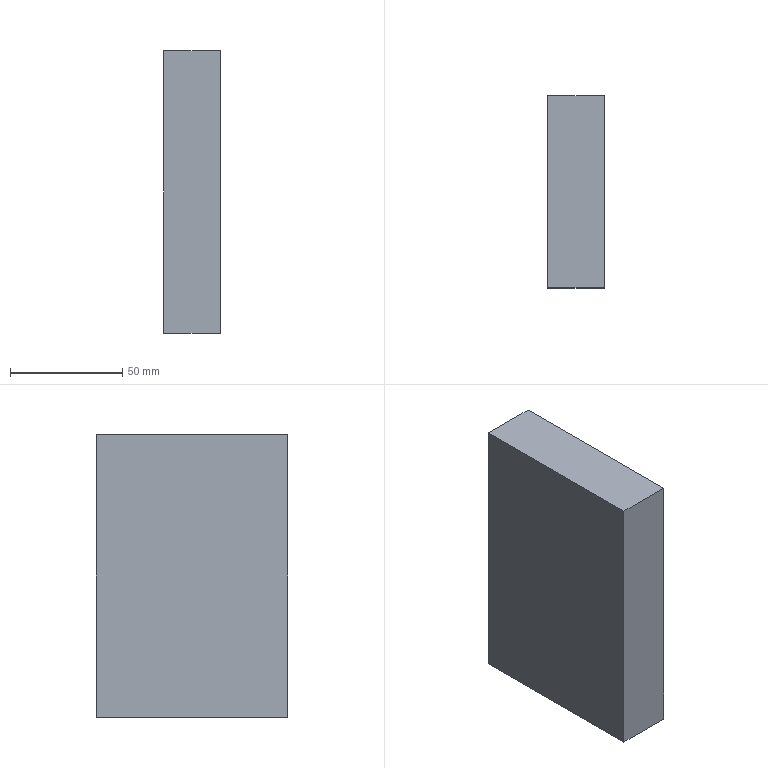Part | SolidWorks | features Extrusion 1 | 1 solid | 6 faces | box 25 x 85.4 x 126 mm | volume 269010 mm3 | plane 6
STEP:
#1=CARTESIAN_POINT('',(-12.5,-42.7,-63.));
#2=VERTEX_POINT('',#1);
#3=CARTESIAN_POINT('',(-12.5,-42.7,63.));
#4=VERTEX_POINT('',#3);
#5=CARTESIAN_POINT('',(-12.5,-42.7,-63.));
#6=DIRECTION('',(0.,0.,1.));
#7=VECTOR('',#6,1000.);
#8=LINE('',#5,#7);
#9=EDGE_CURVE('',#2,#4,#8,.T.);
#10=ORIENTED_EDGE('',*,*,#9,.T.);
#11=CARTESIAN_POINT('',(-12.5,42.7,63.));
#12=VERTEX_POINT('',#11);
#13=CARTESIAN_POINT('',(-12.5,42.7,63.));
#14=DIRECTION('',(0.,-1.,0.));
#15=VECTOR('',#14,1000.);
#16=LINE('',#13,#15);
#17=EDGE_CURVE('',#12,#4,#16,.T.);
#18=ORIENTED_EDGE('',*,*,#17,.F.);
#19=CARTESIAN_POINT('',(-12.5,42.7,-63.));
#20=VERTEX_POINT('',#19);
#21=CARTESIAN_POINT('',(-12.5,42.7,-63.));
#22=DIRECTION('',(0.,0.,1.));
#23=VECTOR('',#22,1000.);
#24=LINE('',#21,#23);
#25=EDGE_CURVE('',#20,#12,#24,.T.);
#26=ORIENTED_EDGE('',*,*,#25,.F.);
#27=CARTESIAN_POINT('',(-12.5,42.7,-63.));
#28=DIRECTION('',(0.,-1.,0.));
#29=VECTOR('',#28,1000.);
#30=LINE('',#27,#29);
#31=EDGE_CURVE('',#20,#2,#30,.T.);
#32=ORIENTED_EDGE('',*,*,#31,.T.);
#33=EDGE_LOOP('',(#10,#18,#26,#32));
#34=FACE_OUTER_BOUND('',#33,.T.);
#35=CARTESIAN_POINT('',(-12.5,42.7,-63.));
#36=DIRECTION('',(1.,0.,0.));
#37=DIRECTION('',(0.,0.,-1.));
#38=AXIS2_PLACEMENT_3D('',#35,#36,#37);
#39=PLANE('',#38);
#40=ADVANCED_FACE('',(#34),#39,.F.);
#41=CARTESIAN_POINT('',(12.5,-42.7,63.));
#42=VERTEX_POINT('',#41);
#43=CARTESIAN_POINT('',(-12.5,-42.7,63.));
#44=DIRECTION('',(1.,0.,0.));
#45=VECTOR('',#44,1000.);
#46=LINE('',#43,#45);
#47=EDGE_CURVE('',#4,#42,#46,.T.);
#48=ORIENTED_EDGE('',*,*,#47,.T.);
#49=CARTESIAN_POINT('',(12.5,42.7,63.));
#50=VERTEX_POINT('',#49);
#51=CARTESIAN_POINT('',(12.5,42.7,63.));
#52=DIRECTION('',(0.,-1.,0.));
#53=VECTOR('',#52,1000.);
#54=LINE('',#51,#53);
#55=EDGE_CURVE('',#50,#42,#54,.T.);
#56=ORIENTED_EDGE('',*,*,#55,.F.);
#57=CARTESIAN_POINT('',(-12.5,42.7,63.));
#58=DIRECTION('',(1.,0.,0.));
#59=VECTOR('',#58,1000.);
#60=LINE('',#57,#59);
#61=EDGE_CURVE('',#12,#50,#60,.T.);
#62=ORIENTED_EDGE('',*,*,#61,.F.);
#63=ORIENTED_EDGE('',*,*,#17,.T.);
#64=EDGE_LOOP('',(#48,#56,#62,#63));
#65=FACE_OUTER_BOUND('',#64,.T.);
#66=CARTESIAN_POINT('',(-12.5,42.7,63.));
#67=DIRECTION('',(0.,0.,-1.));
#68=DIRECTION('',(-1.,0.,0.));
#69=AXIS2_PLACEMENT_3D('',#66,#67,#68);
#70=PLANE('',#69);
#71=ADVANCED_FACE('',(#65),#70,.F.);
#72=CARTESIAN_POINT('',(12.5,-42.7,-63.));
#73=VERTEX_POINT('',#72);
#74=CARTESIAN_POINT('',(12.5,-42.7,-63.));
#75=DIRECTION('',(0.,0.,-1.));
#76=VECTOR('',#75,1000.);
#77=LINE('',#74,#76);
#78=EDGE_CURVE('',#42,#73,#77,.T.);
#79=ORIENTED_EDGE('',*,*,#78,.T.);
#80=CARTESIAN_POINT('',(12.5,42.7,-63.));
#81=VERTEX_POINT('',#80);
#82=CARTESIAN_POINT('',(12.5,42.7,-63.));
#83=DIRECTION('',(0.,-1.,0.));
#84=VECTOR('',#83,1000.);
#85=LINE('',#82,#84);
#86=EDGE_CURVE('',#81,#73,#85,.T.);
#87=ORIENTED_EDGE('',*,*,#86,.F.);
#88=CARTESIAN_POINT('',(12.5,42.7,-63.));
#89=DIRECTION('',(0.,0.,-1.));
#90=VECTOR('',#89,1000.);
#91=LINE('',#88,#90);
#92=EDGE_CURVE('',#50,#81,#91,.T.);
#93=ORIENTED_EDGE('',*,*,#92,.F.);
#94=ORIENTED_EDGE('',*,*,#55,.T.);
#95=EDGE_LOOP('',(#79,#87,#93,#94));
#96=FACE_OUTER_BOUND('',#95,.T.);
#97=CARTESIAN_POINT('',(12.5,42.7,-63.));
#98=DIRECTION('',(-1.,0.,0.));
#99=DIRECTION('',(0.,0.,1.));
#100=AXIS2_PLACEMENT_3D('',#97,#98,#99);
#101=PLANE('',#100);
#102=ADVANCED_FACE('',(#96),#101,.F.);
#103=CARTESIAN_POINT('',(-12.5,-42.7,-63.));
#104=DIRECTION('',(-1.,0.,0.));
#105=VECTOR('',#104,1000.);
#106=LINE('',#103,#105);
#107=EDGE_CURVE('',#73,#2,#106,.T.);
#108=ORIENTED_EDGE('',*,*,#107,.T.);
#109=ORIENTED_EDGE('',*,*,#31,.F.);
#110=CARTESIAN_POINT('',(-12.5,42.7,-63.));
#111=DIRECTION('',(-1.,0.,0.));
#112=VECTOR('',#111,1000.);
#113=LINE('',#110,#112);
#114=EDGE_CURVE('',#81,#20,#113,.T.);
#115=ORIENTED_EDGE('',*,*,#114,.F.);
#116=ORIENTED_EDGE('',*,*,#86,.T.);
#117=EDGE_LOOP('',(#108,#109,#115,#116));
#118=FACE_OUTER_BOUND('',#117,.T.);
#119=CARTESIAN_POINT('',(-12.5,42.7,-63.));
#120=DIRECTION('',(0.,0.,1.));
#121=DIRECTION('',(1.,0.,0.));
#122=AXIS2_PLACEMENT_3D('',#119,#120,#121);
#123=PLANE('',#122);
#124=ADVANCED_FACE('',(#118),#123,.F.);
#125=ORIENTED_EDGE('',*,*,#25,.T.);
#126=ORIENTED_EDGE('',*,*,#61,.T.);
#127=ORIENTED_EDGE('',*,*,#92,.T.);
#128=ORIENTED_EDGE('',*,*,#114,.T.);
#129=EDGE_LOOP('',(#125,#126,#127,#128));
#130=FACE_OUTER_BOUND('',#129,.T.);
#131=CARTESIAN_POINT('',(0.,42.7,0.));
#132=DIRECTION('',(0.,1.,0.));
#133=DIRECTION('',(0.,0.,1.));
#134=AXIS2_PLACEMENT_3D('',#131,#132,#133);
#135=PLANE('',#134);
#136=ADVANCED_FACE('',(#130),#135,.T.);
#137=ORIENTED_EDGE('',*,*,#9,.F.);
#138=ORIENTED_EDGE('',*,*,#107,.F.);
#139=ORIENTED_EDGE('',*,*,#78,.F.);
#140=ORIENTED_EDGE('',*,*,#47,.F.);
#141=EDGE_LOOP('',(#137,#138,#139,#140));
#142=FACE_OUTER_BOUND('',#141,.T.);
#143=CARTESIAN_POINT('',(0.,-42.7,0.));
#144=DIRECTION('',(0.,1.,0.));
#145=DIRECTION('',(0.,0.,1.));
#146=AXIS2_PLACEMENT_3D('',#143,#144,#145);
#147=PLANE('',#146);
#148=ADVANCED_FACE('',(#142),#147,.F.);
#149=CLOSED_SHELL('',(#40,#71,#102,#124,#136,#148));
#150=MANIFOLD_SOLID_BREP('',#149);
#151=CARTESIAN_POINT('',(0.,0.,0.));
#152=DIRECTION('',(0.,0.,1.));
#153=DIRECTION('',(1.,0.,0.));
#154=AXIS2_PLACEMENT_3D('',#151,#152,#153);
#155=(LENGTH_UNIT()NAMED_UNIT(*)SI_UNIT(.MILLI.,.METRE.));
#156=UNCERTAINTY_MEASURE_WITH_UNIT(LENGTH_MEASURE(0.00001),#155,'','');
#157=(NAMED_UNIT(*)PLANE_ANGLE_UNIT()SI_UNIT($,.RADIAN.));
#158=(NAMED_UNIT(*)SI_UNIT($,.STERADIAN.)SOLID_ANGLE_UNIT());
#159=(GEOMETRIC_REPRESENTATION_CONTEXT(3)GLOBAL_UNCERTAINTY_ASSIGNED_CONTEXT((#156))GLOBAL_UNIT_ASSIGNED_CONTEXT((#155,#157,#158))REPRESENTATION_CONTEXT('',''));
#160=ADVANCED_BREP_SHAPE_REPRESENTATION('',(#150,#154),#159);